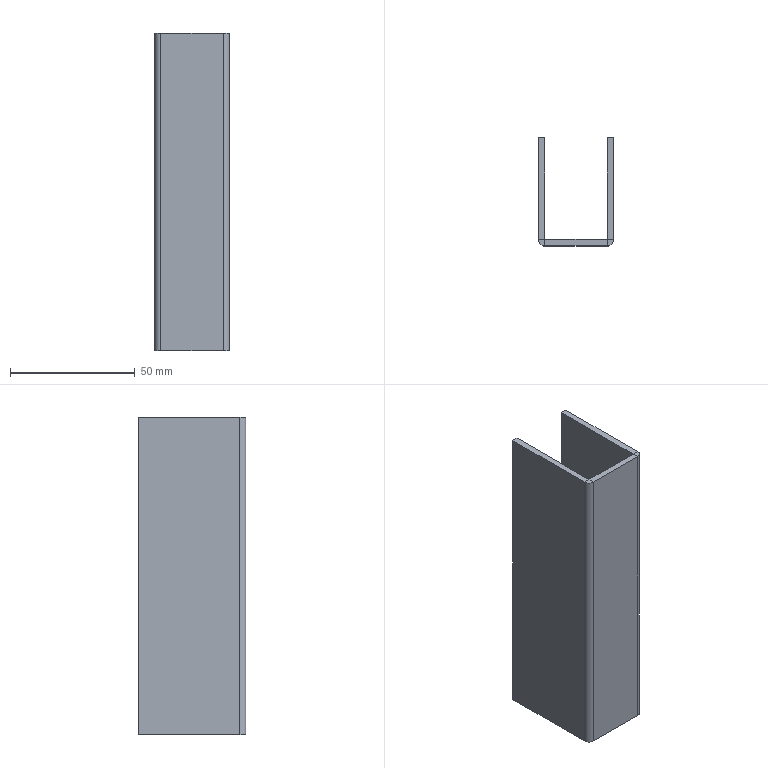Part | NX | features solid 2 | 1 solid | 16 faces | box 30 x 43.21 x 127 mm | volume 35035 mm3 | plane 14 | cylinder 2 | commonest cylinder face diameters 5 x2
STEP:
#1=CARTESIAN_POINT('',(-97.5,-43.21,-1069.5));
#2=VERTEX_POINT('',#1);
#3=CARTESIAN_POINT('',(-97.5,-45.71,-1069.5));
#4=VERTEX_POINT('',#3);
#5=CARTESIAN_POINT('',(-97.5,-43.21,-1069.5));
#6=DIRECTION('',(0.,-1.,0.));
#7=VECTOR('',#6,1000.);
#8=LINE('',#5,#7);
#9=EDGE_CURVE('',#2,#4,#8,.T.);
#10=ORIENTED_EDGE('',*,*,#9,.F.);
#11=CARTESIAN_POINT('',(-100.,-43.21,-1069.5));
#12=VERTEX_POINT('',#11);
#13=CARTESIAN_POINT('',(-97.5,-43.21,-1069.5));
#14=DIRECTION('',(-1.,0.,0.));
#15=VECTOR('',#14,1000.);
#16=LINE('',#13,#15);
#17=EDGE_CURVE('',#2,#12,#16,.T.);
#18=ORIENTED_EDGE('',*,*,#17,.T.);
#19=CARTESIAN_POINT('',(-97.5,-43.21,-1069.5));
#20=DIRECTION('',(0.,0.,-1.));
#21=DIRECTION('',(0.,-1.,0.));
#22=AXIS2_PLACEMENT_3D('',#19,#20,#21);
#23=CIRCLE('',#22,2.5);
#24=EDGE_CURVE('',#4,#12,#23,.T.);
#25=ORIENTED_EDGE('',*,*,#24,.F.);
#26=EDGE_LOOP('',(#10,#18,#25));
#27=FACE_BOUND('',#26,.T.);
#28=CARTESIAN_POINT('',(-98.384,-44.094,-1069.5));
#29=DIRECTION('',(0.,0.,-1.));
#30=DIRECTION('',(0.,1.,0.));
#31=AXIS2_PLACEMENT_3D('',#28,#29,#30);
#32=PLANE('',#31);
#33=ADVANCED_FACE('',(#27),#32,.F.);
#34=ORIENTED_EDGE('',*,*,#24,.T.);
#35=CARTESIAN_POINT('',(-100.,-43.21,-1196.5));
#36=VERTEX_POINT('',#35);
#37=CARTESIAN_POINT('',(-100.,-43.21,-1196.5));
#38=DIRECTION('',(0.,0.,1.));
#39=VECTOR('',#38,1000.);
#40=LINE('',#37,#39);
#41=EDGE_CURVE('',#36,#12,#40,.T.);
#42=ORIENTED_EDGE('',*,*,#41,.F.);
#43=CARTESIAN_POINT('',(-97.5,-45.71,-1196.5));
#44=VERTEX_POINT('',#43);
#45=CARTESIAN_POINT('',(-97.5,-43.21,-1196.5));
#46=DIRECTION('',(0.,0.,1.));
#47=DIRECTION('',(-1.,0.,0.));
#48=AXIS2_PLACEMENT_3D('',#45,#46,#47);
#49=CIRCLE('',#48,2.5);
#50=EDGE_CURVE('',#36,#44,#49,.T.);
#51=ORIENTED_EDGE('',*,*,#50,.T.);
#52=CARTESIAN_POINT('',(-97.5,-45.71,-1069.5));
#53=DIRECTION('',(0.,0.,-1.));
#54=VECTOR('',#53,1000.);
#55=LINE('',#52,#54);
#56=EDGE_CURVE('',#4,#44,#55,.T.);
#57=ORIENTED_EDGE('',*,*,#56,.F.);
#58=EDGE_LOOP('',(#34,#42,#51,#57));
#59=FACE_BOUND('',#58,.T.);
#60=CARTESIAN_POINT('',(-97.5,-43.21,-1574.153));
#61=DIRECTION('',(0.,0.,1.));
#62=DIRECTION('',(1.,0.,0.));
#63=AXIS2_PLACEMENT_3D('',#60,#61,#62);
#64=CYLINDRICAL_SURFACE('',#63,2.5);
#65=ADVANCED_FACE('',(#59),#64,.T.);
#66=CARTESIAN_POINT('',(-72.5,-45.71,-1069.5));
#67=VERTEX_POINT('',#66);
#68=CARTESIAN_POINT('',(-97.5,-45.71,-1069.5));
#69=DIRECTION('',(1.,0.,0.));
#70=VECTOR('',#69,1000.);
#71=LINE('',#68,#70);
#72=EDGE_CURVE('',#4,#67,#71,.T.);
#73=ORIENTED_EDGE('',*,*,#72,.F.);
#74=ORIENTED_EDGE('',*,*,#56,.T.);
#75=CARTESIAN_POINT('',(-72.5,-45.71,-1196.5));
#76=VERTEX_POINT('',#75);
#77=CARTESIAN_POINT('',(-97.5,-45.71,-1196.5));
#78=DIRECTION('',(1.,0.,0.));
#79=VECTOR('',#78,1000.);
#80=LINE('',#77,#79);
#81=EDGE_CURVE('',#44,#76,#80,.T.);
#82=ORIENTED_EDGE('',*,*,#81,.T.);
#83=CARTESIAN_POINT('',(-72.5,-45.71,-1196.5));
#84=DIRECTION('',(0.,0.,1.));
#85=VECTOR('',#84,1000.);
#86=LINE('',#83,#85);
#87=EDGE_CURVE('',#76,#67,#86,.T.);
#88=ORIENTED_EDGE('',*,*,#87,.T.);
#89=EDGE_LOOP('',(#73,#74,#82,#88));
#90=FACE_BOUND('',#89,.T.);
#91=CARTESIAN_POINT('',(-70.,-45.71,-1069.5));
#92=DIRECTION('',(0.,-1.,0.));
#93=DIRECTION('',(1.,0.,0.));
#94=AXIS2_PLACEMENT_3D('',#91,#92,#93);
#95=PLANE('',#94);
#96=ADVANCED_FACE('',(#90),#95,.T.);
#97=CARTESIAN_POINT('',(-70.,-43.21,-1069.5));
#98=VERTEX_POINT('',#97);
#99=CARTESIAN_POINT('',(-72.5,-43.21,-1069.5));
#100=DIRECTION('',(0.,0.,-1.));
#101=DIRECTION('',(1.,0.,0.));
#102=AXIS2_PLACEMENT_3D('',#99,#100,#101);
#103=CIRCLE('',#102,2.5);
#104=EDGE_CURVE('',#98,#67,#103,.T.);
#105=ORIENTED_EDGE('',*,*,#104,.T.);
#106=ORIENTED_EDGE('',*,*,#87,.F.);
#107=CARTESIAN_POINT('',(-70.,-43.21,-1196.5));
#108=VERTEX_POINT('',#107);
#109=CARTESIAN_POINT('',(-72.5,-43.21,-1196.5));
#110=DIRECTION('',(0.,0.,1.));
#111=DIRECTION('',(0.,-1.,0.));
#112=AXIS2_PLACEMENT_3D('',#109,#110,#111);
#113=CIRCLE('',#112,2.5);
#114=EDGE_CURVE('',#76,#108,#113,.T.);
#115=ORIENTED_EDGE('',*,*,#114,.T.);
#116=CARTESIAN_POINT('',(-70.,-43.21,-1069.5));
#117=DIRECTION('',(0.,0.,-1.));
#118=VECTOR('',#117,1000.);
#119=LINE('',#116,#118);
#120=EDGE_CURVE('',#98,#108,#119,.T.);
#121=ORIENTED_EDGE('',*,*,#120,.F.);
#122=EDGE_LOOP('',(#105,#106,#115,#121));
#123=FACE_BOUND('',#122,.T.);
#124=CARTESIAN_POINT('',(-72.5,-43.21,-1574.153));
#125=DIRECTION('',(0.,0.,1.));
#126=DIRECTION('',(0.,1.,0.));
#127=AXIS2_PLACEMENT_3D('',#124,#125,#126);
#128=CYLINDRICAL_SURFACE('',#127,2.5);
#129=ADVANCED_FACE('',(#123),#128,.T.);
#130=CARTESIAN_POINT('',(-70.,-2.5,-1196.5));
#131=VERTEX_POINT('',#130);
#132=CARTESIAN_POINT('',(-70.,-43.21,-1196.5));
#133=DIRECTION('',(0.,1.,0.));
#134=VECTOR('',#133,1000.);
#135=LINE('',#132,#134);
#136=EDGE_CURVE('',#108,#131,#135,.T.);
#137=ORIENTED_EDGE('',*,*,#136,.T.);
#138=CARTESIAN_POINT('',(-70.,-2.5,-1069.5));
#139=VERTEX_POINT('',#138);
#140=CARTESIAN_POINT('',(-70.,-2.5,-1196.5));
#141=DIRECTION('',(0.,0.,1.));
#142=VECTOR('',#141,1000.);
#143=LINE('',#140,#142);
#144=EDGE_CURVE('',#131,#139,#143,.T.);
#145=ORIENTED_EDGE('',*,*,#144,.T.);
#146=CARTESIAN_POINT('',(-70.,-43.21,-1069.5));
#147=DIRECTION('',(0.,1.,0.));
#148=VECTOR('',#147,1000.);
#149=LINE('',#146,#148);
#150=EDGE_CURVE('',#98,#139,#149,.T.);
#151=ORIENTED_EDGE('',*,*,#150,.F.);
#152=ORIENTED_EDGE('',*,*,#120,.T.);
#153=EDGE_LOOP('',(#137,#145,#151,#152));
#154=FACE_BOUND('',#153,.T.);
#155=CARTESIAN_POINT('',(-70.,-2.5,-1069.5));
#156=DIRECTION('',(1.,0.,0.));
#157=DIRECTION('',(0.,1.,0.));
#158=AXIS2_PLACEMENT_3D('',#155,#156,#157);
#159=PLANE('',#158);
#160=ADVANCED_FACE('',(#154),#159,.T.);
#161=ORIENTED_EDGE('',*,*,#150,.T.);
#162=CARTESIAN_POINT('',(-72.5,-2.5,-1069.5));
#163=VERTEX_POINT('',#162);
#164=CARTESIAN_POINT('',(-72.5,-2.5,-1069.5));
#165=DIRECTION('',(1.,0.,0.));
#166=VECTOR('',#165,1000.);
#167=LINE('',#164,#166);
#168=EDGE_CURVE('',#163,#139,#167,.T.);
#169=ORIENTED_EDGE('',*,*,#168,.F.);
#170=CARTESIAN_POINT('',(-72.5,-43.21,-1069.5));
#171=VERTEX_POINT('',#170);
#172=CARTESIAN_POINT('',(-72.5,-43.21,-1069.5));
#173=DIRECTION('',(0.,1.,0.));
#174=VECTOR('',#173,1000.);
#175=LINE('',#172,#174);
#176=EDGE_CURVE('',#171,#163,#175,.T.);
#177=ORIENTED_EDGE('',*,*,#176,.F.);
#178=CARTESIAN_POINT('',(-72.5,-43.21,-1069.5));
#179=DIRECTION('',(1.,0.,0.));
#180=VECTOR('',#179,1000.);
#181=LINE('',#178,#180);
#182=EDGE_CURVE('',#171,#98,#181,.T.);
#183=ORIENTED_EDGE('',*,*,#182,.T.);
#184=EDGE_LOOP('',(#161,#169,#177,#183));
#185=FACE_BOUND('',#184,.T.);
#186=CARTESIAN_POINT('',(-71.25,-23.48,-1069.5));
#187=DIRECTION('',(0.,0.,1.));
#188=DIRECTION('',(0.,1.,0.));
#189=AXIS2_PLACEMENT_3D('',#186,#187,#188);
#190=PLANE('',#189);
#191=ADVANCED_FACE('',(#185),#190,.T.);
#192=ORIENTED_EDGE('',*,*,#182,.F.);
#193=CARTESIAN_POINT('',(-72.5,-43.21,-1069.5));
#194=DIRECTION('',(0.,-1.,0.));
#195=VECTOR('',#194,1000.);
#196=LINE('',#193,#195);
#197=EDGE_CURVE('',#171,#67,#196,.T.);
#198=ORIENTED_EDGE('',*,*,#197,.T.);
#199=ORIENTED_EDGE('',*,*,#104,.F.);
#200=EDGE_LOOP('',(#192,#198,#199));
#201=FACE_BOUND('',#200,.T.);
#202=CARTESIAN_POINT('',(-71.616,-44.094,-1069.5));
#203=DIRECTION('',(0.,0.,-1.));
#204=DIRECTION('',(-1.,0.,0.));
#205=AXIS2_PLACEMENT_3D('',#202,#203,#204);
#206=PLANE('',#205);
#207=ADVANCED_FACE('',(#201),#206,.F.);
#208=ORIENTED_EDGE('',*,*,#72,.T.);
#209=ORIENTED_EDGE('',*,*,#197,.F.);
#210=CARTESIAN_POINT('',(-97.5,-43.21,-1069.5));
#211=DIRECTION('',(1.,0.,0.));
#212=VECTOR('',#211,1000.);
#213=LINE('',#210,#212);
#214=EDGE_CURVE('',#2,#171,#213,.T.);
#215=ORIENTED_EDGE('',*,*,#214,.F.);
#216=ORIENTED_EDGE('',*,*,#9,.T.);
#217=EDGE_LOOP('',(#208,#209,#215,#216));
#218=FACE_BOUND('',#217,.T.);
#219=CARTESIAN_POINT('',(-85.,-44.46,-1069.5));
#220=DIRECTION('',(0.,0.,1.));
#221=DIRECTION('',(1.,0.,0.));
#222=AXIS2_PLACEMENT_3D('',#219,#220,#221);
#223=PLANE('',#222);
#224=ADVANCED_FACE('',(#218),#223,.T.);
#225=CARTESIAN_POINT('',(-97.5,-43.21,-1196.5));
#226=VERTEX_POINT('',#225);
#227=CARTESIAN_POINT('',(-72.5,-43.21,-1196.5));
#228=VERTEX_POINT('',#227);
#229=CARTESIAN_POINT('',(-97.5,-43.21,-1196.5));
#230=DIRECTION('',(1.,0.,0.));
#231=VECTOR('',#230,1000.);
#232=LINE('',#229,#231);
#233=EDGE_CURVE('',#226,#228,#232,.T.);
#234=ORIENTED_EDGE('',*,*,#233,.F.);
#235=CARTESIAN_POINT('',(-97.5,-43.21,-1069.5));
#236=DIRECTION('',(0.,0.,-1.));
#237=VECTOR('',#236,1000.);
#238=LINE('',#235,#237);
#239=EDGE_CURVE('',#2,#226,#238,.T.);
#240=ORIENTED_EDGE('',*,*,#239,.F.);
#241=ORIENTED_EDGE('',*,*,#214,.T.);
#242=CARTESIAN_POINT('',(-72.5,-43.21,-1069.5));
#243=DIRECTION('',(0.,0.,-1.));
#244=VECTOR('',#243,1000.);
#245=LINE('',#242,#244);
#246=EDGE_CURVE('',#171,#228,#245,.T.);
#247=ORIENTED_EDGE('',*,*,#246,.T.);
#248=EDGE_LOOP('',(#234,#240,#241,#247));
#249=FACE_BOUND('',#248,.T.);
#250=CARTESIAN_POINT('',(-70.,-43.21,-1069.5));
#251=DIRECTION('',(0.,-1.,0.));
#252=DIRECTION('',(1.,0.,0.));
#253=AXIS2_PLACEMENT_3D('',#250,#251,#252);
#254=PLANE('',#253);
#255=ADVANCED_FACE('',(#249),#254,.F.);
#256=ORIENTED_EDGE('',*,*,#176,.T.);
#257=CARTESIAN_POINT('',(-72.5,-2.5,-1196.5));
#258=VERTEX_POINT('',#257);
#259=CARTESIAN_POINT('',(-72.5,-2.5,-1196.5));
#260=DIRECTION('',(0.,0.,1.));
#261=VECTOR('',#260,1000.);
#262=LINE('',#259,#261);
#263=EDGE_CURVE('',#258,#163,#262,.T.);
#264=ORIENTED_EDGE('',*,*,#263,.F.);
#265=CARTESIAN_POINT('',(-72.5,-43.21,-1196.5));
#266=DIRECTION('',(0.,1.,0.));
#267=VECTOR('',#266,1000.);
#268=LINE('',#265,#267);
#269=EDGE_CURVE('',#228,#258,#268,.T.);
#270=ORIENTED_EDGE('',*,*,#269,.F.);
#271=ORIENTED_EDGE('',*,*,#246,.F.);
#272=EDGE_LOOP('',(#256,#264,#270,#271));
#273=FACE_BOUND('',#272,.T.);
#274=CARTESIAN_POINT('',(-72.5,-2.5,-1069.5));
#275=DIRECTION('',(1.,0.,0.));
#276=DIRECTION('',(0.,1.,0.));
#277=AXIS2_PLACEMENT_3D('',#274,#275,#276);
#278=PLANE('',#277);
#279=ADVANCED_FACE('',(#273),#278,.F.);
#280=CARTESIAN_POINT('',(-72.5,-2.5,-1196.5));
#281=DIRECTION('',(1.,0.,0.));
#282=VECTOR('',#281,1000.);
#283=LINE('',#280,#282);
#284=EDGE_CURVE('',#258,#131,#283,.T.);
#285=ORIENTED_EDGE('',*,*,#284,.T.);
#286=ORIENTED_EDGE('',*,*,#136,.F.);
#287=ORIENTED_EDGE('',*,*,#114,.F.);
#288=ORIENTED_EDGE('',*,*,#81,.F.);
#289=ORIENTED_EDGE('',*,*,#50,.F.);
#290=CARTESIAN_POINT('',(-100.,-2.5,-1196.5));
#291=VERTEX_POINT('',#290);
#292=CARTESIAN_POINT('',(-100.,-2.5,-1196.5));
#293=DIRECTION('',(0.,-1.,0.));
#294=VECTOR('',#293,1000.);
#295=LINE('',#292,#294);
#296=EDGE_CURVE('',#291,#36,#295,.T.);
#297=ORIENTED_EDGE('',*,*,#296,.F.);
#298=CARTESIAN_POINT('',(-97.5,-2.5,-1196.5));
#299=VERTEX_POINT('',#298);
#300=CARTESIAN_POINT('',(-97.5,-2.5,-1196.5));
#301=DIRECTION('',(-1.,0.,0.));
#302=VECTOR('',#301,1000.);
#303=LINE('',#300,#302);
#304=EDGE_CURVE('',#299,#291,#303,.T.);
#305=ORIENTED_EDGE('',*,*,#304,.F.);
#306=CARTESIAN_POINT('',(-97.5,-2.5,-1196.5));
#307=DIRECTION('',(0.,-1.,0.));
#308=VECTOR('',#307,1000.);
#309=LINE('',#306,#308);
#310=EDGE_CURVE('',#299,#226,#309,.T.);
#311=ORIENTED_EDGE('',*,*,#310,.T.);
#312=ORIENTED_EDGE('',*,*,#233,.T.);
#313=ORIENTED_EDGE('',*,*,#269,.T.);
#314=EDGE_LOOP('',(#285,#286,#287,#288,#289,#297,#305,#311,#312,#313));
#315=FACE_BOUND('',#314,.T.);
#316=CARTESIAN_POINT('',(-71.25,-23.48,-1196.5));
#317=DIRECTION('',(0.,0.,1.));
#318=DIRECTION('',(0.,1.,0.));
#319=AXIS2_PLACEMENT_3D('',#316,#317,#318);
#320=PLANE('',#319);
#321=ADVANCED_FACE('',(#315),#320,.F.);
#322=ORIENTED_EDGE('',*,*,#310,.F.);
#323=CARTESIAN_POINT('',(-97.5,-2.5,-1069.5));
#324=VERTEX_POINT('',#323);
#325=CARTESIAN_POINT('',(-97.5,-2.5,-1196.5));
#326=DIRECTION('',(0.,0.,1.));
#327=VECTOR('',#326,1000.);
#328=LINE('',#325,#327);
#329=EDGE_CURVE('',#299,#324,#328,.T.);
#330=ORIENTED_EDGE('',*,*,#329,.T.);
#331=CARTESIAN_POINT('',(-97.5,-2.5,-1069.5));
#332=DIRECTION('',(0.,-1.,0.));
#333=VECTOR('',#332,1000.);
#334=LINE('',#331,#333);
#335=EDGE_CURVE('',#324,#2,#334,.T.);
#336=ORIENTED_EDGE('',*,*,#335,.T.);
#337=ORIENTED_EDGE('',*,*,#239,.T.);
#338=EDGE_LOOP('',(#322,#330,#336,#337));
#339=FACE_BOUND('',#338,.T.);
#340=CARTESIAN_POINT('',(-97.5,-45.71,-1069.5));
#341=DIRECTION('',(-1.,0.,0.));
#342=DIRECTION('',(0.,-1.,0.));
#343=AXIS2_PLACEMENT_3D('',#340,#341,#342);
#344=PLANE('',#343);
#345=ADVANCED_FACE('',(#339),#344,.F.);
#346=ORIENTED_EDGE('',*,*,#335,.F.);
#347=CARTESIAN_POINT('',(-100.,-2.5,-1069.5));
#348=VERTEX_POINT('',#347);
#349=CARTESIAN_POINT('',(-97.5,-2.5,-1069.5));
#350=DIRECTION('',(-1.,0.,0.));
#351=VECTOR('',#350,1000.);
#352=LINE('',#349,#351);
#353=EDGE_CURVE('',#324,#348,#352,.T.);
#354=ORIENTED_EDGE('',*,*,#353,.T.);
#355=CARTESIAN_POINT('',(-100.,-2.5,-1069.5));
#356=DIRECTION('',(0.,-1.,0.));
#357=VECTOR('',#356,1000.);
#358=LINE('',#355,#357);
#359=EDGE_CURVE('',#348,#12,#358,.T.);
#360=ORIENTED_EDGE('',*,*,#359,.T.);
#361=ORIENTED_EDGE('',*,*,#17,.F.);
#362=EDGE_LOOP('',(#346,#354,#360,#361));
#363=FACE_BOUND('',#362,.T.);
#364=CARTESIAN_POINT('',(-98.75,-23.48,-1069.5));
#365=DIRECTION('',(0.,0.,1.));
#366=DIRECTION('',(0.,-1.,0.));
#367=AXIS2_PLACEMENT_3D('',#364,#365,#366);
#368=PLANE('',#367);
#369=ADVANCED_FACE('',(#363),#368,.T.);
#370=ORIENTED_EDGE('',*,*,#359,.F.);
#371=CARTESIAN_POINT('',(-100.,-2.5,-1196.5));
#372=DIRECTION('',(0.,0.,1.));
#373=VECTOR('',#372,1000.);
#374=LINE('',#371,#373);
#375=EDGE_CURVE('',#291,#348,#374,.T.);
#376=ORIENTED_EDGE('',*,*,#375,.F.);
#377=ORIENTED_EDGE('',*,*,#296,.T.);
#378=ORIENTED_EDGE('',*,*,#41,.T.);
#379=EDGE_LOOP('',(#370,#376,#377,#378));
#380=FACE_BOUND('',#379,.T.);
#381=CARTESIAN_POINT('',(-100.,-45.71,-1069.5));
#382=DIRECTION('',(-1.,0.,0.));
#383=DIRECTION('',(0.,-1.,0.));
#384=AXIS2_PLACEMENT_3D('',#381,#382,#383);
#385=PLANE('',#384);
#386=ADVANCED_FACE('',(#380),#385,.T.);
#387=ORIENTED_EDGE('',*,*,#353,.F.);
#388=ORIENTED_EDGE('',*,*,#329,.F.);
#389=ORIENTED_EDGE('',*,*,#304,.T.);
#390=ORIENTED_EDGE('',*,*,#375,.T.);
#391=EDGE_LOOP('',(#387,#388,#389,#390));
#392=FACE_BOUND('',#391,.T.);
#393=CARTESIAN_POINT('',(-98.75,-2.5,-1177.));
#394=DIRECTION('',(0.,1.,0.));
#395=DIRECTION('',(0.,0.,1.));
#396=AXIS2_PLACEMENT_3D('',#393,#394,#395);
#397=PLANE('',#396);
#398=ADVANCED_FACE('',(#392),#397,.T.);
#399=ORIENTED_EDGE('',*,*,#284,.F.);
#400=ORIENTED_EDGE('',*,*,#263,.T.);
#401=ORIENTED_EDGE('',*,*,#168,.T.);
#402=ORIENTED_EDGE('',*,*,#144,.F.);
#403=EDGE_LOOP('',(#399,#400,#401,#402));
#404=FACE_BOUND('',#403,.T.);
#405=CARTESIAN_POINT('',(-71.25,-2.5,-1177.));
#406=DIRECTION('',(0.,-1.,0.));
#407=DIRECTION('',(0.,0.,1.));
#408=AXIS2_PLACEMENT_3D('',#405,#406,#407);
#409=PLANE('',#408);
#410=ADVANCED_FACE('',(#404),#409,.F.);
#411=CLOSED_SHELL('',(#33,#65,#96,#129,#160,#191,#207,#224,#255,#279,#321,#345,#369,#386,#398,#410));
#412=MANIFOLD_SOLID_BREP('',#411);
#413=(LENGTH_UNIT()NAMED_UNIT(*)SI_UNIT(.MILLI.,.METRE.));
#414=UNCERTAINTY_MEASURE_WITH_UNIT(LENGTH_MEASURE(0.00001),#413,'','');
#415=(NAMED_UNIT(*)PLANE_ANGLE_UNIT()SI_UNIT($,.RADIAN.));
#416=(NAMED_UNIT(*)SI_UNIT($,.STERADIAN.)SOLID_ANGLE_UNIT());
#417=(GEOMETRIC_REPRESENTATION_CONTEXT(3)GLOBAL_UNCERTAINTY_ASSIGNED_CONTEXT((#414))GLOBAL_UNIT_ASSIGNED_CONTEXT((#413,#415,#416))REPRESENTATION_CONTEXT('',''));
#418=ADVANCED_BREP_SHAPE_REPRESENTATION('',(#412),#417);